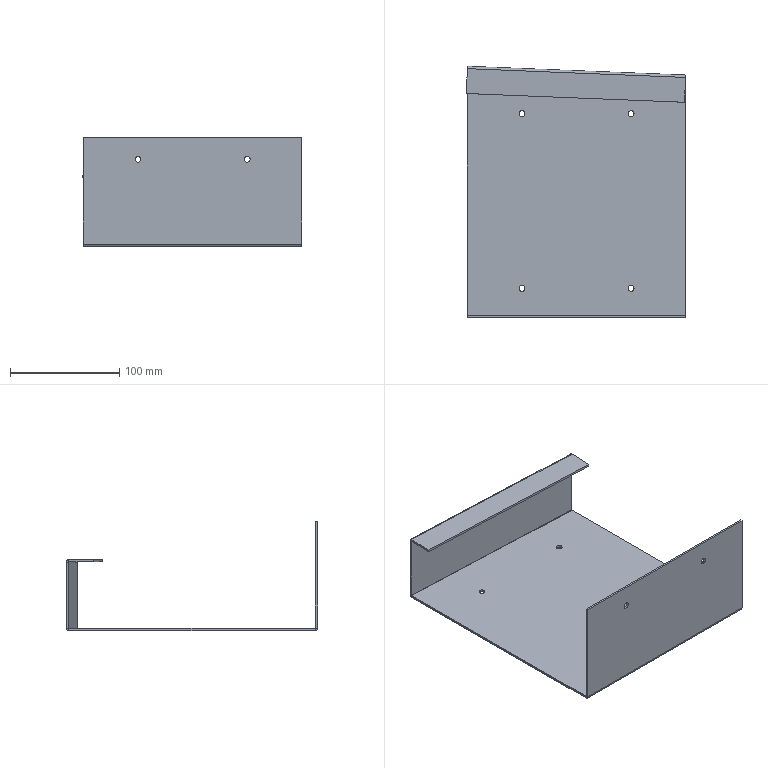Part | STEP file | TS-S22 | 1 solid | 43 faces | box 201.003 x 230.402 x 100 mm | volume 163289 mm3 | plane 24 | cylinder 18 | spline 1 | commonest cylinder face diameters 5.4 x12 0.4 x3 4.4 x3